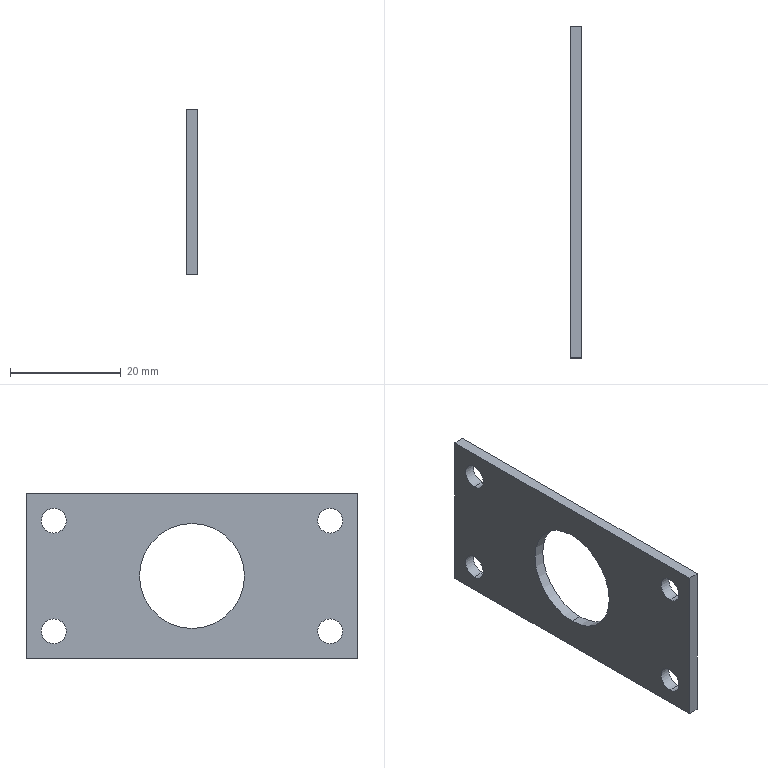Part | STEP file | 06-07 Bearing cover plate | 1 solid | 16 faces | box 2 x 60 x 30 mm | volume 2906 mm3 | cylinder 10 | plane 6 | commonest cylinder face diameters 4.5 x8 19 x2
STEP:
#1=CARTESIAN_POINT('',(0.,0.,0.));
#2=DIRECTION('',(0.,0.,1.));
#3=DIRECTION('',(1.,0.,0.));
#4=AXIS2_PLACEMENT_3D('',#1,#2,#3);
#5=CARTESIAN_POINT('',(2.,-24.996,-7.75));
#6=VERTEX_POINT('',#5);
#7=CARTESIAN_POINT('',(0.,-24.996,-7.75));
#8=VERTEX_POINT('',#7);
#9=CARTESIAN_POINT('',(2.,-24.996,-7.75));
#10=DIRECTION('',(-1.,0.,0.));
#11=VECTOR('',#10,1.);
#12=LINE('',#9,#11);
#13=CARTESIAN_POINT('',(2.,-24.996,-10.));
#14=DIRECTION('',(-1.,0.,0.));
#15=DIRECTION('',(0.,0.,1.));
#16=AXIS2_PLACEMENT_3D('',#13,#14,#15);
#17=CYLINDRICAL_SURFACE('',#16,2.25);
#18=CARTESIAN_POINT('',(6.283,0.));
#19=DIRECTION('',(0.,1.));
#20=VECTOR('',#19,1.);
#21=LINE('',#18,#20);
#22=(GEOMETRIC_REPRESENTATION_CONTEXT(2)PARAMETRIC_REPRESENTATION_CONTEXT()REPRESENTATION_CONTEXT('',''));
#23=DEFINITIONAL_REPRESENTATION('',(#21),#22);
#24=PCURVE('',#17,#23);
#25=CARTESIAN_POINT('',(2.,-24.996,-10.));
#26=DIRECTION('',(-1.,0.,0.));
#27=DIRECTION('',(0.,0.,1.));
#28=AXIS2_PLACEMENT_3D('',#25,#26,#27);
#29=CYLINDRICAL_SURFACE('',#28,2.25);
#30=CARTESIAN_POINT('',(0.,0.));
#31=DIRECTION('',(0.,1.));
#32=VECTOR('',#31,1.);
#33=LINE('',#30,#32);
#34=(GEOMETRIC_REPRESENTATION_CONTEXT(2)PARAMETRIC_REPRESENTATION_CONTEXT()REPRESENTATION_CONTEXT('',''));
#35=DEFINITIONAL_REPRESENTATION('',(#33),#34);
#36=PCURVE('',#29,#35);
#37=SURFACE_CURVE('',#12,(#24,#36),.PCURVE_S1.);
#38=EDGE_CURVE('',#6,#8,#37,.T.);
#39=ORIENTED_EDGE('',*,*,#38,.T.);
#40=CARTESIAN_POINT('',(0.,-24.996,-12.25));
#41=VERTEX_POINT('',#40);
#42=CARTESIAN_POINT('',(0.,-24.996,-10.));
#43=DIRECTION('',(-1.,0.,0.));
#44=DIRECTION('',(0.,0.,1.));
#45=AXIS2_PLACEMENT_3D('',#42,#43,#44);
#46=CIRCLE('',#45,2.25);
#47=CARTESIAN_POINT('',(0.,2.));
#48=DIRECTION('',(1.,0.));
#49=VECTOR('',#48,1.);
#50=LINE('',#47,#49);
#51=(GEOMETRIC_REPRESENTATION_CONTEXT(2)PARAMETRIC_REPRESENTATION_CONTEXT()REPRESENTATION_CONTEXT('',''));
#52=DEFINITIONAL_REPRESENTATION('',(#50),#51);
#53=PCURVE('',#17,#52);
#54=CARTESIAN_POINT('',(0.,-30.,15.));
#55=DIRECTION('',(1.,0.,0.));
#56=DIRECTION('',(0.,0.,-1.));
#57=AXIS2_PLACEMENT_3D('',#54,#55,#56);
#58=PLANE('',#57);
#59=CARTESIAN_POINT('',(22.75,5.004));
#60=CARTESIAN_POINT('',(22.75,8.901));
#61=CARTESIAN_POINT('',(26.125,6.952));
#62=CARTESIAN_POINT('',(29.5,5.004));
#63=CARTESIAN_POINT('',(26.125,3.055));
#64=CARTESIAN_POINT('',(22.75,1.107));
#65=CARTESIAN_POINT('',(22.75,5.004));
#66=(BOUNDED_CURVE()B_SPLINE_CURVE(2,(#59,#60,#61,#62,#63,#64,#65),.UNSPECIFIED.,.T.,.F.)B_SPLINE_CURVE_WITH_KNOTS((1,2,2,2,2,1),(-2.094,0.,2.094,4.189,6.283,8.378),.UNSPECIFIED.)CURVE()GEOMETRIC_REPRESENTATION_ITEM()RATIONAL_B_SPLINE_CURVE((1.,0.5,1.,0.5,1.,0.5,1.))REPRESENTATION_ITEM(''));
#67=(GEOMETRIC_REPRESENTATION_CONTEXT(2)PARAMETRIC_REPRESENTATION_CONTEXT()REPRESENTATION_CONTEXT('',''));
#68=DEFINITIONAL_REPRESENTATION('',(#66),#67);
#69=PCURVE('',#58,#68);
#70=SURFACE_CURVE('',#46,(#53,#69),.PCURVE_S1.);
#71=EDGE_CURVE('',#41,#8,#70,.T.);
#72=ORIENTED_EDGE('',*,*,#71,.F.);
#73=CARTESIAN_POINT('',(2.,-24.996,-12.25));
#74=VERTEX_POINT('',#73);
#75=CARTESIAN_POINT('',(2.,-24.996,-12.25));
#76=DIRECTION('',(-1.,0.,0.));
#77=VECTOR('',#76,1.);
#78=LINE('',#75,#77);
#79=CARTESIAN_POINT('',(3.142,0.));
#80=DIRECTION('',(0.,1.));
#81=VECTOR('',#80,1.);
#82=LINE('',#79,#81);
#83=(GEOMETRIC_REPRESENTATION_CONTEXT(2)PARAMETRIC_REPRESENTATION_CONTEXT()REPRESENTATION_CONTEXT('',''));
#84=DEFINITIONAL_REPRESENTATION('',(#82),#83);
#85=PCURVE('',#17,#84);
#86=CARTESIAN_POINT('',(3.142,0.));
#87=DIRECTION('',(0.,1.));
#88=VECTOR('',#87,1.);
#89=LINE('',#86,#88);
#90=(GEOMETRIC_REPRESENTATION_CONTEXT(2)PARAMETRIC_REPRESENTATION_CONTEXT()REPRESENTATION_CONTEXT('',''));
#91=DEFINITIONAL_REPRESENTATION('',(#89),#90);
#92=PCURVE('',#29,#91);
#93=SURFACE_CURVE('',#78,(#85,#92),.PCURVE_S1.);
#94=EDGE_CURVE('',#74,#41,#93,.T.);
#95=ORIENTED_EDGE('',*,*,#94,.F.);
#96=CARTESIAN_POINT('',(2.,-24.996,-10.));
#97=DIRECTION('',(1.,0.,0.));
#98=DIRECTION('',(0.,0.,1.));
#99=AXIS2_PLACEMENT_3D('',#96,#97,#98);
#100=CIRCLE('',#99,2.25);
#101=CARTESIAN_POINT('',(6.283,0.));
#102=DIRECTION('',(-1.,0.));
#103=VECTOR('',#102,1.);
#104=LINE('',#101,#103);
#105=(GEOMETRIC_REPRESENTATION_CONTEXT(2)PARAMETRIC_REPRESENTATION_CONTEXT()REPRESENTATION_CONTEXT('',''));
#106=DEFINITIONAL_REPRESENTATION('',(#104),#105);
#107=PCURVE('',#17,#106);
#108=CARTESIAN_POINT('',(2.,-30.,15.));
#109=DIRECTION('',(1.,0.,0.));
#110=DIRECTION('',(0.,0.,-1.));
#111=AXIS2_PLACEMENT_3D('',#108,#109,#110);
#112=PLANE('',#111);
#113=CARTESIAN_POINT('',(25.,5.004));
#114=DIRECTION('',(-1.,0.));
#115=AXIS2_PLACEMENT_2D('',#113,#114);
#116=CIRCLE('',#115,2.25);
#117=(GEOMETRIC_REPRESENTATION_CONTEXT(2)PARAMETRIC_REPRESENTATION_CONTEXT()REPRESENTATION_CONTEXT('',''));
#118=DEFINITIONAL_REPRESENTATION('',(#116),#117);
#119=PCURVE('',#112,#118);
#120=SURFACE_CURVE('',#100,(#107,#119),.PCURVE_S1.);
#121=EDGE_CURVE('',#6,#74,#120,.T.);
#122=ORIENTED_EDGE('',*,*,#121,.F.);
#123=EDGE_LOOP('',(#39,#72,#95,#122));
#124=FACE_BOUND('',#123,.F.);
#125=ADVANCED_FACE('',(#124),#17,.F.);
#126=CARTESIAN_POINT('',(2.,25.004,-7.75));
#127=VERTEX_POINT('',#126);
#128=CARTESIAN_POINT('',(0.,25.004,-7.75));
#129=VERTEX_POINT('',#128);
#130=CARTESIAN_POINT('',(2.,25.004,-7.75));
#131=DIRECTION('',(-1.,0.,0.));
#132=VECTOR('',#131,1.);
#133=LINE('',#130,#132);
#134=CARTESIAN_POINT('',(2.,25.004,-10.));
#135=DIRECTION('',(-1.,0.,0.));
#136=DIRECTION('',(0.,0.,1.));
#137=AXIS2_PLACEMENT_3D('',#134,#135,#136);
#138=CYLINDRICAL_SURFACE('',#137,2.25);
#139=CARTESIAN_POINT('',(6.283,0.));
#140=DIRECTION('',(0.,1.));
#141=VECTOR('',#140,1.);
#142=LINE('',#139,#141);
#143=(GEOMETRIC_REPRESENTATION_CONTEXT(2)PARAMETRIC_REPRESENTATION_CONTEXT()REPRESENTATION_CONTEXT('',''));
#144=DEFINITIONAL_REPRESENTATION('',(#142),#143);
#145=PCURVE('',#138,#144);
#146=CARTESIAN_POINT('',(2.,25.004,-10.));
#147=DIRECTION('',(-1.,0.,0.));
#148=DIRECTION('',(0.,0.,1.));
#149=AXIS2_PLACEMENT_3D('',#146,#147,#148);
#150=CYLINDRICAL_SURFACE('',#149,2.25);
#151=CARTESIAN_POINT('',(0.,0.));
#152=DIRECTION('',(0.,1.));
#153=VECTOR('',#152,1.);
#154=LINE('',#151,#153);
#155=(GEOMETRIC_REPRESENTATION_CONTEXT(2)PARAMETRIC_REPRESENTATION_CONTEXT()REPRESENTATION_CONTEXT('',''));
#156=DEFINITIONAL_REPRESENTATION('',(#154),#155);
#157=PCURVE('',#150,#156);
#158=SURFACE_CURVE('',#133,(#145,#157),.PCURVE_S1.);
#159=EDGE_CURVE('',#127,#129,#158,.T.);
#160=ORIENTED_EDGE('',*,*,#159,.T.);
#161=CARTESIAN_POINT('',(0.,25.004,-12.25));
#162=VERTEX_POINT('',#161);
#163=CARTESIAN_POINT('',(0.,25.004,-10.));
#164=DIRECTION('',(-1.,0.,0.));
#165=DIRECTION('',(0.,0.,1.));
#166=AXIS2_PLACEMENT_3D('',#163,#164,#165);
#167=CIRCLE('',#166,2.25);
#168=CARTESIAN_POINT('',(0.,2.));
#169=DIRECTION('',(1.,0.));
#170=VECTOR('',#169,1.);
#171=LINE('',#168,#170);
#172=(GEOMETRIC_REPRESENTATION_CONTEXT(2)PARAMETRIC_REPRESENTATION_CONTEXT()REPRESENTATION_CONTEXT('',''));
#173=DEFINITIONAL_REPRESENTATION('',(#171),#172);
#174=PCURVE('',#138,#173);
#175=CARTESIAN_POINT('',(22.75,55.004));
#176=CARTESIAN_POINT('',(22.75,58.901));
#177=CARTESIAN_POINT('',(26.125,56.952));
#178=CARTESIAN_POINT('',(29.5,55.004));
#179=CARTESIAN_POINT('',(26.125,53.055));
#180=CARTESIAN_POINT('',(22.75,51.107));
#181=CARTESIAN_POINT('',(22.75,55.004));
#182=(BOUNDED_CURVE()B_SPLINE_CURVE(2,(#175,#176,#177,#178,#179,#180,#181),.UNSPECIFIED.,.T.,.F.)B_SPLINE_CURVE_WITH_KNOTS((1,2,2,2,2,1),(-2.094,0.,2.094,4.189,6.283,8.378),.UNSPECIFIED.)CURVE()GEOMETRIC_REPRESENTATION_ITEM()RATIONAL_B_SPLINE_CURVE((1.,0.5,1.,0.5,1.,0.5,1.))REPRESENTATION_ITEM(''));
#183=(GEOMETRIC_REPRESENTATION_CONTEXT(2)PARAMETRIC_REPRESENTATION_CONTEXT()REPRESENTATION_CONTEXT('',''));
#184=DEFINITIONAL_REPRESENTATION('',(#182),#183);
#185=PCURVE('',#58,#184);
#186=SURFACE_CURVE('',#167,(#174,#185),.PCURVE_S1.);
#187=EDGE_CURVE('',#162,#129,#186,.T.);
#188=ORIENTED_EDGE('',*,*,#187,.F.);
#189=CARTESIAN_POINT('',(2.,25.004,-12.25));
#190=VERTEX_POINT('',#189);
#191=CARTESIAN_POINT('',(2.,25.004,-12.25));
#192=DIRECTION('',(-1.,0.,0.));
#193=VECTOR('',#192,1.);
#194=LINE('',#191,#193);
#195=CARTESIAN_POINT('',(3.142,0.));
#196=DIRECTION('',(0.,1.));
#197=VECTOR('',#196,1.);
#198=LINE('',#195,#197);
#199=(GEOMETRIC_REPRESENTATION_CONTEXT(2)PARAMETRIC_REPRESENTATION_CONTEXT()REPRESENTATION_CONTEXT('',''));
#200=DEFINITIONAL_REPRESENTATION('',(#198),#199);
#201=PCURVE('',#138,#200);
#202=CARTESIAN_POINT('',(3.142,0.));
#203=DIRECTION('',(0.,1.));
#204=VECTOR('',#203,1.);
#205=LINE('',#202,#204);
#206=(GEOMETRIC_REPRESENTATION_CONTEXT(2)PARAMETRIC_REPRESENTATION_CONTEXT()REPRESENTATION_CONTEXT('',''));
#207=DEFINITIONAL_REPRESENTATION('',(#205),#206);
#208=PCURVE('',#150,#207);
#209=SURFACE_CURVE('',#194,(#201,#208),.PCURVE_S1.);
#210=EDGE_CURVE('',#190,#162,#209,.T.);
#211=ORIENTED_EDGE('',*,*,#210,.F.);
#212=CARTESIAN_POINT('',(2.,25.004,-10.));
#213=DIRECTION('',(-1.,0.,0.));
#214=DIRECTION('',(0.,0.,1.));
#215=AXIS2_PLACEMENT_3D('',#212,#213,#214);
#216=CIRCLE('',#215,2.25);
#217=CARTESIAN_POINT('',(0.,0.));
#218=DIRECTION('',(1.,0.));
#219=VECTOR('',#218,1.);
#220=LINE('',#217,#219);
#221=(GEOMETRIC_REPRESENTATION_CONTEXT(2)PARAMETRIC_REPRESENTATION_CONTEXT()REPRESENTATION_CONTEXT('',''));
#222=DEFINITIONAL_REPRESENTATION('',(#220),#221);
#223=PCURVE('',#138,#222);
#224=CARTESIAN_POINT('',(22.75,55.004));
#225=CARTESIAN_POINT('',(22.75,58.901));
#226=CARTESIAN_POINT('',(26.125,56.952));
#227=CARTESIAN_POINT('',(29.5,55.004));
#228=CARTESIAN_POINT('',(26.125,53.055));
#229=CARTESIAN_POINT('',(22.75,51.107));
#230=CARTESIAN_POINT('',(22.75,55.004));
#231=(BOUNDED_CURVE()B_SPLINE_CURVE(2,(#224,#225,#226,#227,#228,#229,#230),.UNSPECIFIED.,.T.,.F.)B_SPLINE_CURVE_WITH_KNOTS((1,2,2,2,2,1),(-2.094,0.,2.094,4.189,6.283,8.378),.UNSPECIFIED.)CURVE()GEOMETRIC_REPRESENTATION_ITEM()RATIONAL_B_SPLINE_CURVE((1.,0.5,1.,0.5,1.,0.5,1.))REPRESENTATION_ITEM(''));
#232=(GEOMETRIC_REPRESENTATION_CONTEXT(2)PARAMETRIC_REPRESENTATION_CONTEXT()REPRESENTATION_CONTEXT('',''));
#233=DEFINITIONAL_REPRESENTATION('',(#231),#232);
#234=PCURVE('',#112,#233);
#235=SURFACE_CURVE('',#216,(#223,#234),.PCURVE_S1.);
#236=EDGE_CURVE('',#190,#127,#235,.T.);
#237=ORIENTED_EDGE('',*,*,#236,.T.);
#238=EDGE_LOOP('',(#160,#188,#211,#237));
#239=FACE_BOUND('',#238,.F.);
#240=ADVANCED_FACE('',(#239),#138,.F.);
#241=CARTESIAN_POINT('',(2.,0.,9.5));
#242=VERTEX_POINT('',#241);
#243=CARTESIAN_POINT('',(0.,0.,9.5));
#244=VERTEX_POINT('',#243);
#245=CARTESIAN_POINT('',(2.,0.,9.5));
#246=DIRECTION('',(-1.,0.,0.));
#247=VECTOR('',#246,1.);
#248=LINE('',#245,#247);
#249=CARTESIAN_POINT('',(2.,0.,0.));
#250=DIRECTION('',(-1.,0.,0.));
#251=DIRECTION('',(0.,0.,1.));
#252=AXIS2_PLACEMENT_3D('',#249,#250,#251);
#253=CYLINDRICAL_SURFACE('',#252,9.5);
#254=CARTESIAN_POINT('',(6.283,0.));
#255=DIRECTION('',(0.,1.));
#256=VECTOR('',#255,1.);
#257=LINE('',#254,#256);
#258=(GEOMETRIC_REPRESENTATION_CONTEXT(2)PARAMETRIC_REPRESENTATION_CONTEXT()REPRESENTATION_CONTEXT('',''));
#259=DEFINITIONAL_REPRESENTATION('',(#257),#258);
#260=PCURVE('',#253,#259);
#261=CARTESIAN_POINT('',(2.,0.,0.));
#262=DIRECTION('',(-1.,0.,0.));
#263=DIRECTION('',(0.,0.,1.));
#264=AXIS2_PLACEMENT_3D('',#261,#262,#263);
#265=CYLINDRICAL_SURFACE('',#264,9.5);
#266=CARTESIAN_POINT('',(0.,0.));
#267=DIRECTION('',(0.,1.));
#268=VECTOR('',#267,1.);
#269=LINE('',#266,#268);
#270=(GEOMETRIC_REPRESENTATION_CONTEXT(2)PARAMETRIC_REPRESENTATION_CONTEXT()REPRESENTATION_CONTEXT('',''));
#271=DEFINITIONAL_REPRESENTATION('',(#269),#270);
#272=PCURVE('',#265,#271);
#273=SURFACE_CURVE('',#248,(#260,#272),.PCURVE_S1.);
#274=EDGE_CURVE('',#242,#244,#273,.T.);
#275=ORIENTED_EDGE('',*,*,#274,.T.);
#276=CARTESIAN_POINT('',(0.,0.,-9.5));
#277=VERTEX_POINT('',#276);
#278=CARTESIAN_POINT('',(0.,0.,0.));
#279=DIRECTION('',(-1.,0.,0.));
#280=DIRECTION('',(0.,0.,1.));
#281=AXIS2_PLACEMENT_3D('',#278,#279,#280);
#282=CIRCLE('',#281,9.5);
#283=CARTESIAN_POINT('',(0.,2.));
#284=DIRECTION('',(1.,0.));
#285=VECTOR('',#284,1.);
#286=LINE('',#283,#285);
#287=(GEOMETRIC_REPRESENTATION_CONTEXT(2)PARAMETRIC_REPRESENTATION_CONTEXT()REPRESENTATION_CONTEXT('',''));
#288=DEFINITIONAL_REPRESENTATION('',(#286),#287);
#289=PCURVE('',#253,#288);
#290=CARTESIAN_POINT('',(5.5,30.));
#291=CARTESIAN_POINT('',(5.5,46.454));
#292=CARTESIAN_POINT('',(19.75,38.227));
#293=CARTESIAN_POINT('',(34.,30.));
#294=CARTESIAN_POINT('',(19.75,21.773));
#295=CARTESIAN_POINT('',(5.5,13.546));
#296=CARTESIAN_POINT('',(5.5,30.));
#297=(BOUNDED_CURVE()B_SPLINE_CURVE(2,(#290,#291,#292,#293,#294,#295,#296),.UNSPECIFIED.,.T.,.F.)B_SPLINE_CURVE_WITH_KNOTS((1,2,2,2,2,1),(-2.094,0.,2.094,4.189,6.283,8.378),.UNSPECIFIED.)CURVE()GEOMETRIC_REPRESENTATION_ITEM()RATIONAL_B_SPLINE_CURVE((1.,0.5,1.,0.5,1.,0.5,1.))REPRESENTATION_ITEM(''));
#298=(GEOMETRIC_REPRESENTATION_CONTEXT(2)PARAMETRIC_REPRESENTATION_CONTEXT()REPRESENTATION_CONTEXT('',''));
#299=DEFINITIONAL_REPRESENTATION('',(#297),#298);
#300=PCURVE('',#58,#299);
#301=SURFACE_CURVE('',#282,(#289,#300),.PCURVE_S1.);
#302=EDGE_CURVE('',#277,#244,#301,.T.);
#303=ORIENTED_EDGE('',*,*,#302,.F.);
#304=CARTESIAN_POINT('',(2.,0.,-9.5));
#305=VERTEX_POINT('',#304);
#306=CARTESIAN_POINT('',(2.,0.,-9.5));
#307=DIRECTION('',(-1.,0.,0.));
#308=VECTOR('',#307,1.);
#309=LINE('',#306,#308);
#310=CARTESIAN_POINT('',(3.142,0.));
#311=DIRECTION('',(0.,1.));
#312=VECTOR('',#311,1.);
#313=LINE('',#310,#312);
#314=(GEOMETRIC_REPRESENTATION_CONTEXT(2)PARAMETRIC_REPRESENTATION_CONTEXT()REPRESENTATION_CONTEXT('',''));
#315=DEFINITIONAL_REPRESENTATION('',(#313),#314);
#316=PCURVE('',#253,#315);
#317=CARTESIAN_POINT('',(3.142,0.));
#318=DIRECTION('',(0.,1.));
#319=VECTOR('',#318,1.);
#320=LINE('',#317,#319);
#321=(GEOMETRIC_REPRESENTATION_CONTEXT(2)PARAMETRIC_REPRESENTATION_CONTEXT()REPRESENTATION_CONTEXT('',''));
#322=DEFINITIONAL_REPRESENTATION('',(#320),#321);
#323=PCURVE('',#265,#322);
#324=SURFACE_CURVE('',#309,(#316,#323),.PCURVE_S1.);
#325=EDGE_CURVE('',#305,#277,#324,.T.);
#326=ORIENTED_EDGE('',*,*,#325,.F.);
#327=CARTESIAN_POINT('',(2.,0.,0.));
#328=DIRECTION('',(-1.,0.,0.));
#329=DIRECTION('',(0.,0.,1.));
#330=AXIS2_PLACEMENT_3D('',#327,#328,#329);
#331=CIRCLE('',#330,9.5);
#332=CARTESIAN_POINT('',(0.,0.));
#333=DIRECTION('',(1.,0.));
#334=VECTOR('',#333,1.);
#335=LINE('',#332,#334);
#336=(GEOMETRIC_REPRESENTATION_CONTEXT(2)PARAMETRIC_REPRESENTATION_CONTEXT()REPRESENTATION_CONTEXT('',''));
#337=DEFINITIONAL_REPRESENTATION('',(#335),#336);
#338=PCURVE('',#253,#337);
#339=CARTESIAN_POINT('',(5.5,30.));
#340=CARTESIAN_POINT('',(5.5,46.454));
#341=CARTESIAN_POINT('',(19.75,38.227));
#342=CARTESIAN_POINT('',(34.,30.));
#343=CARTESIAN_POINT('',(19.75,21.773));
#344=CARTESIAN_POINT('',(5.5,13.546));
#345=CARTESIAN_POINT('',(5.5,30.));
#346=(BOUNDED_CURVE()B_SPLINE_CURVE(2,(#339,#340,#341,#342,#343,#344,#345),.UNSPECIFIED.,.T.,.F.)B_SPLINE_CURVE_WITH_KNOTS((1,2,2,2,2,1),(-2.094,0.,2.094,4.189,6.283,8.378),.UNSPECIFIED.)CURVE()GEOMETRIC_REPRESENTATION_ITEM()RATIONAL_B_SPLINE_CURVE((1.,0.5,1.,0.5,1.,0.5,1.))REPRESENTATION_ITEM(''));
#347=(GEOMETRIC_REPRESENTATION_CONTEXT(2)PARAMETRIC_REPRESENTATION_CONTEXT()REPRESENTATION_CONTEXT('',''));
#348=DEFINITIONAL_REPRESENTATION('',(#346),#347);
#349=PCURVE('',#112,#348);
#350=SURFACE_CURVE('',#331,(#338,#349),.PCURVE_S1.);
#351=EDGE_CURVE('',#305,#242,#350,.T.);
#352=ORIENTED_EDGE('',*,*,#351,.T.);
#353=EDGE_LOOP('',(#275,#303,#326,#352));
#354=FACE_BOUND('',#353,.F.);
#355=ADVANCED_FACE('',(#354),#253,.F.);
#356=CARTESIAN_POINT('',(2.,25.004,12.25));
#357=VERTEX_POINT('',#356);
#358=CARTESIAN_POINT('',(0.,25.004,12.25));
#359=VERTEX_POINT('',#358);
#360=CARTESIAN_POINT('',(2.,25.004,12.25));
#361=DIRECTION('',(-1.,0.,0.));
#362=VECTOR('',#361,1.);
#363=LINE('',#360,#362);
#364=CARTESIAN_POINT('',(2.,25.004,10.));
#365=DIRECTION('',(-1.,0.,0.));
#366=DIRECTION('',(0.,0.,1.));
#367=AXIS2_PLACEMENT_3D('',#364,#365,#366);
#368=CYLINDRICAL_SURFACE('',#367,2.25);
#369=CARTESIAN_POINT('',(6.283,0.));
#370=DIRECTION('',(0.,1.));
#371=VECTOR('',#370,1.);
#372=LINE('',#369,#371);
#373=(GEOMETRIC_REPRESENTATION_CONTEXT(2)PARAMETRIC_REPRESENTATION_CONTEXT()REPRESENTATION_CONTEXT('',''));
#374=DEFINITIONAL_REPRESENTATION('',(#372),#373);
#375=PCURVE('',#368,#374);
#376=CARTESIAN_POINT('',(2.,25.004,10.));
#377=DIRECTION('',(-1.,0.,0.));
#378=DIRECTION('',(0.,0.,1.));
#379=AXIS2_PLACEMENT_3D('',#376,#377,#378);
#380=CYLINDRICAL_SURFACE('',#379,2.25);
#381=CARTESIAN_POINT('',(0.,0.));
#382=DIRECTION('',(0.,1.));
#383=VECTOR('',#382,1.);
#384=LINE('',#381,#383);
#385=(GEOMETRIC_REPRESENTATION_CONTEXT(2)PARAMETRIC_REPRESENTATION_CONTEXT()REPRESENTATION_CONTEXT('',''));
#386=DEFINITIONAL_REPRESENTATION('',(#384),#385);
#387=PCURVE('',#380,#386);
#388=SURFACE_CURVE('',#363,(#375,#387),.PCURVE_S1.);
#389=EDGE_CURVE('',#357,#359,#388,.T.);
#390=ORIENTED_EDGE('',*,*,#389,.T.);
#391=CARTESIAN_POINT('',(0.,25.004,7.75));
#392=VERTEX_POINT('',#391);
#393=CARTESIAN_POINT('',(0.,25.004,10.));
#394=DIRECTION('',(-1.,0.,0.));
#395=DIRECTION('',(0.,0.,1.));
#396=AXIS2_PLACEMENT_3D('',#393,#394,#395);
#397=CIRCLE('',#396,2.25);
#398=CARTESIAN_POINT('',(0.,2.));
#399=DIRECTION('',(1.,0.));
#400=VECTOR('',#399,1.);
#401=LINE('',#398,#400);
#402=(GEOMETRIC_REPRESENTATION_CONTEXT(2)PARAMETRIC_REPRESENTATION_CONTEXT()REPRESENTATION_CONTEXT('',''));
#403=DEFINITIONAL_REPRESENTATION('',(#401),#402);
#404=PCURVE('',#368,#403);
#405=CARTESIAN_POINT('',(2.75,55.004));
#406=CARTESIAN_POINT('',(2.75,58.901));
#407=CARTESIAN_POINT('',(6.125,56.952));
#408=CARTESIAN_POINT('',(9.5,55.004));
#409=CARTESIAN_POINT('',(6.125,53.055));
#410=CARTESIAN_POINT('',(2.75,51.107));
#411=CARTESIAN_POINT('',(2.75,55.004));
#412=(BOUNDED_CURVE()B_SPLINE_CURVE(2,(#405,#406,#407,#408,#409,#410,#411),.UNSPECIFIED.,.T.,.F.)B_SPLINE_CURVE_WITH_KNOTS((1,2,2,2,2,1),(-2.094,0.,2.094,4.189,6.283,8.378),.UNSPECIFIED.)CURVE()GEOMETRIC_REPRESENTATION_ITEM()RATIONAL_B_SPLINE_CURVE((1.,0.5,1.,0.5,1.,0.5,1.))REPRESENTATION_ITEM(''));
#413=(GEOMETRIC_REPRESENTATION_CONTEXT(2)PARAMETRIC_REPRESENTATION_CONTEXT()REPRESENTATION_CONTEXT('',''));
#414=DEFINITIONAL_REPRESENTATION('',(#412),#413);
#415=PCURVE('',#58,#414);
#416=SURFACE_CURVE('',#397,(#404,#415),.PCURVE_S1.);
#417=EDGE_CURVE('',#392,#359,#416,.T.);
#418=ORIENTED_EDGE('',*,*,#417,.F.);
#419=CARTESIAN_POINT('',(2.,25.004,7.75));
#420=VERTEX_POINT('',#419);
#421=CARTESIAN_POINT('',(2.,25.004,7.75));
#422=DIRECTION('',(-1.,0.,0.));
#423=VECTOR('',#422,1.);
#424=LINE('',#421,#423);
#425=CARTESIAN_POINT('',(3.142,0.));
#426=DIRECTION('',(0.,1.));
#427=VECTOR('',#426,1.);
#428=LINE('',#425,#427);
#429=(GEOMETRIC_REPRESENTATION_CONTEXT(2)PARAMETRIC_REPRESENTATION_CONTEXT()REPRESENTATION_CONTEXT('',''));
#430=DEFINITIONAL_REPRESENTATION('',(#428),#429);
#431=PCURVE('',#368,#430);
#432=CARTESIAN_POINT('',(3.142,0.));
#433=DIRECTION('',(0.,1.));
#434=VECTOR('',#433,1.);
#435=LINE('',#432,#434);
#436=(GEOMETRIC_REPRESENTATION_CONTEXT(2)PARAMETRIC_REPRESENTATION_CONTEXT()REPRESENTATION_CONTEXT('',''));
#437=DEFINITIONAL_REPRESENTATION('',(#435),#436);
#438=PCURVE('',#380,#437);
#439=SURFACE_CURVE('',#424,(#431,#438),.PCURVE_S1.);
#440=EDGE_CURVE('',#420,#392,#439,.T.);
#441=ORIENTED_EDGE('',*,*,#440,.F.);
#442=CARTESIAN_POINT('',(2.,25.004,10.));
#443=DIRECTION('',(-1.,0.,0.));
#444=DIRECTION('',(0.,0.,1.));
#445=AXIS2_PLACEMENT_3D('',#442,#443,#444);
#446=CIRCLE('',#445,2.25);
#447=CARTESIAN_POINT('',(0.,0.));
#448=DIRECTION('',(1.,0.));
#449=VECTOR('',#448,1.);
#450=LINE('',#447,#449);
#451=(GEOMETRIC_REPRESENTATION_CONTEXT(2)PARAMETRIC_REPRESENTATION_CONTEXT()REPRESENTATION_CONTEXT('',''));
#452=DEFINITIONAL_REPRESENTATION('',(#450),#451);
#453=PCURVE('',#368,#452);
#454=CARTESIAN_POINT('',(2.75,55.004));
#455=CARTESIAN_POINT('',(2.75,58.901));
#456=CARTESIAN_POINT('',(6.125,56.952));
#457=CARTESIAN_POINT('',(9.5,55.004));
#458=CARTESIAN_POINT('',(6.125,53.055));
#459=CARTESIAN_POINT('',(2.75,51.107));
#460=CARTESIAN_POINT('',(2.75,55.004));
#461=(BOUNDED_CURVE()B_SPLINE_CURVE(2,(#454,#455,#456,#457,#458,#459,#460),.UNSPECIFIED.,.T.,.F.)B_SPLINE_CURVE_WITH_KNOTS((1,2,2,2,2,1),(-2.094,0.,2.094,4.189,6.283,8.378),.UNSPECIFIED.)CURVE()GEOMETRIC_REPRESENTATION_ITEM()RATIONAL_B_SPLINE_CURVE((1.,0.5,1.,0.5,1.,0.5,1.))REPRESENTATION_ITEM(''));
#462=(GEOMETRIC_REPRESENTATION_CONTEXT(2)PARAMETRIC_REPRESENTATION_CONTEXT()REPRESENTATION_CONTEXT('',''));
#463=DEFINITIONAL_REPRESENTATION('',(#461),#462);
#464=PCURVE('',#112,#463);
#465=SURFACE_CURVE('',#446,(#453,#464),.PCURVE_S1.);
#466=EDGE_CURVE('',#420,#357,#465,.T.);
#467=ORIENTED_EDGE('',*,*,#466,.T.);
#468=EDGE_LOOP('',(#390,#418,#441,#467));
#469=FACE_BOUND('',#468,.F.);
#470=ADVANCED_FACE('',(#469),#368,.F.);
#471=CARTESIAN_POINT('',(2.,-24.996,12.25));
#472=VERTEX_POINT('',#471);
#473=CARTESIAN_POINT('',(0.,-24.996,12.25));
#474=VERTEX_POINT('',#473);
#475=CARTESIAN_POINT('',(2.,-24.996,12.25));
#476=DIRECTION('',(-1.,0.,0.));
#477=VECTOR('',#476,1.);
#478=LINE('',#475,#477);
#479=CARTESIAN_POINT('',(2.,-24.996,10.));
#480=DIRECTION('',(-1.,0.,0.));
#481=DIRECTION('',(0.,0.,1.));
#482=AXIS2_PLACEMENT_3D('',#479,#480,#481);
#483=CYLINDRICAL_SURFACE('',#482,2.25);
#484=CARTESIAN_POINT('',(6.283,0.));
#485=DIRECTION('',(0.,1.));
#486=VECTOR('',#485,1.);
#487=LINE('',#484,#486);
#488=(GEOMETRIC_REPRESENTATION_CONTEXT(2)PARAMETRIC_REPRESENTATION_CONTEXT()REPRESENTATION_CONTEXT('',''));
#489=DEFINITIONAL_REPRESENTATION('',(#487),#488);
#490=PCURVE('',#483,#489);
#491=CARTESIAN_POINT('',(2.,-24.996,10.));
#492=DIRECTION('',(-1.,0.,0.));
#493=DIRECTION('',(0.,0.,1.));
#494=AXIS2_PLACEMENT_3D('',#491,#492,#493);
#495=CYLINDRICAL_SURFACE('',#494,2.25);
#496=CARTESIAN_POINT('',(0.,0.));
#497=DIRECTION('',(0.,1.));
#498=VECTOR('',#497,1.);
#499=LINE('',#496,#498);
#500=(GEOMETRIC_REPRESENTATION_CONTEXT(2)PARAMETRIC_REPRESENTATION_CONTEXT()REPRESENTATION_CONTEXT('',''));
#501=DEFINITIONAL_REPRESENTATION('',(#499),#500);
#502=PCURVE('',#495,#501);
#503=SURFACE_CURVE('',#478,(#490,#502),.PCURVE_S1.);
#504=EDGE_CURVE('',#472,#474,#503,.T.);
#505=ORIENTED_EDGE('',*,*,#504,.T.);
#506=CARTESIAN_POINT('',(0.,-24.996,7.75));
#507=VERTEX_POINT('',#506);
#508=CARTESIAN_POINT('',(0.,-24.996,10.));
#509=DIRECTION('',(-1.,0.,0.));
#510=DIRECTION('',(0.,0.,1.));
#511=AXIS2_PLACEMENT_3D('',#508,#509,#510);
#512=CIRCLE('',#511,2.25);
#513=CARTESIAN_POINT('',(0.,2.));
#514=DIRECTION('',(1.,0.));
#515=VECTOR('',#514,1.);
#516=LINE('',#513,#515);
#517=(GEOMETRIC_REPRESENTATION_CONTEXT(2)PARAMETRIC_REPRESENTATION_CONTEXT()REPRESENTATION_CONTEXT('',''));
#518=DEFINITIONAL_REPRESENTATION('',(#516),#517);
#519=PCURVE('',#483,#518);
#520=CARTESIAN_POINT('',(2.75,5.004));
#521=CARTESIAN_POINT('',(2.75,8.901));
#522=CARTESIAN_POINT('',(6.125,6.952));
#523=CARTESIAN_POINT('',(9.5,5.004));
#524=CARTESIAN_POINT('',(6.125,3.055));
#525=CARTESIAN_POINT('',(2.75,1.107));
#526=CARTESIAN_POINT('',(2.75,5.004));
#527=(BOUNDED_CURVE()B_SPLINE_CURVE(2,(#520,#521,#522,#523,#524,#525,#526),.UNSPECIFIED.,.T.,.F.)B_SPLINE_CURVE_WITH_KNOTS((1,2,2,2,2,1),(-2.094,0.,2.094,4.189,6.283,8.378),.UNSPECIFIED.)CURVE()GEOMETRIC_REPRESENTATION_ITEM()RATIONAL_B_SPLINE_CURVE((1.,0.5,1.,0.5,1.,0.5,1.))REPRESENTATION_ITEM(''));
#528=(GEOMETRIC_REPRESENTATION_CONTEXT(2)PARAMETRIC_REPRESENTATION_CONTEXT()REPRESENTATION_CONTEXT('',''));
#529=DEFINITIONAL_REPRESENTATION('',(#527),#528);
#530=PCURVE('',#58,#529);
#531=SURFACE_CURVE('',#512,(#519,#530),.PCURVE_S1.);
#532=EDGE_CURVE('',#507,#474,#531,.T.);
#533=ORIENTED_EDGE('',*,*,#532,.F.);
#534=CARTESIAN_POINT('',(2.,-24.996,7.75));
#535=VERTEX_POINT('',#534);
#536=CARTESIAN_POINT('',(2.,-24.996,7.75));
#537=DIRECTION('',(-1.,0.,0.));
#538=VECTOR('',#537,1.);
#539=LINE('',#536,#538);
#540=CARTESIAN_POINT('',(3.142,0.));
#541=DIRECTION('',(0.,1.));
#542=VECTOR('',#541,1.);
#543=LINE('',#540,#542);
#544=(GEOMETRIC_REPRESENTATION_CONTEXT(2)PARAMETRIC_REPRESENTATION_CONTEXT()REPRESENTATION_CONTEXT('',''));
#545=DEFINITIONAL_REPRESENTATION('',(#543),#544);
#546=PCURVE('',#483,#545);
#547=CARTESIAN_POINT('',(3.142,0.));
#548=DIRECTION('',(0.,1.));
#549=VECTOR('',#548,1.);
#550=LINE('',#547,#549);
#551=(GEOMETRIC_REPRESENTATION_CONTEXT(2)PARAMETRIC_REPRESENTATION_CONTEXT()REPRESENTATION_CONTEXT('',''));
#552=DEFINITIONAL_REPRESENTATION('',(#550),#551);
#553=PCURVE('',#495,#552);
#554=SURFACE_CURVE('',#539,(#546,#553),.PCURVE_S1.);
#555=EDGE_CURVE('',#535,#507,#554,.T.);
#556=ORIENTED_EDGE('',*,*,#555,.F.);
#557=CARTESIAN_POINT('',(2.,-24.996,10.));
#558=DIRECTION('',(-1.,0.,0.));
#559=DIRECTION('',(0.,0.,1.));
#560=AXIS2_PLACEMENT_3D('',#557,#558,#559);
#561=CIRCLE('',#560,2.25);
#562=CARTESIAN_POINT('',(0.,0.));
#563=DIRECTION('',(1.,0.));
#564=VECTOR('',#563,1.);
#565=LINE('',#562,#564);
#566=(GEOMETRIC_REPRESENTATION_CONTEXT(2)PARAMETRIC_REPRESENTATION_CONTEXT()REPRESENTATION_CONTEXT('',''));
#567=DEFINITIONAL_REPRESENTATION('',(#565),#566);
#568=PCURVE('',#483,#567);
#569=CARTESIAN_POINT('',(2.75,5.004));
#570=CARTESIAN_POINT('',(2.75,8.901));
#571=CARTESIAN_POINT('',(6.125,6.952));
#572=CARTESIAN_POINT('',(9.5,5.004));
#573=CARTESIAN_POINT('',(6.125,3.055));
#574=CARTESIAN_POINT('',(2.75,1.107));
#575=CARTESIAN_POINT('',(2.75,5.004));
#576=(BOUNDED_CURVE()B_SPLINE_CURVE(2,(#569,#570,#571,#572,#573,#574,#575),.UNSPECIFIED.,.T.,.F.)B_SPLINE_CURVE_WITH_KNOTS((1,2,2,2,2,1),(-2.094,0.,2.094,4.189,6.283,8.378),.UNSPECIFIED.)CURVE()GEOMETRIC_REPRESENTATION_ITEM()RATIONAL_B_SPLINE_CURVE((1.,0.5,1.,0.5,1.,0.5,1.))REPRESENTATION_ITEM(''));
#577=(GEOMETRIC_REPRESENTATION_CONTEXT(2)PARAMETRIC_REPRESENTATION_CONTEXT()REPRESENTATION_CONTEXT('',''));
#578=DEFINITIONAL_REPRESENTATION('',(#576),#577);
#579=PCURVE('',#112,#578);
#580=SURFACE_CURVE('',#561,(#568,#579),.PCURVE_S1.);
#581=EDGE_CURVE('',#535,#472,#580,.T.);
#582=ORIENTED_EDGE('',*,*,#581,.T.);
#583=EDGE_LOOP('',(#505,#533,#556,#582));
#584=FACE_BOUND('',#583,.F.);
#585=ADVANCED_FACE('',(#584),#483,.F.);
#586=CARTESIAN_POINT('',(0.,-24.996,-10.));
#587=DIRECTION('',(-1.,0.,0.));
#588=DIRECTION('',(0.,0.,1.));
#589=AXIS2_PLACEMENT_3D('',#586,#587,#588);
#590=CIRCLE('',#589,2.25);
#591=CARTESIAN_POINT('',(0.,2.));
#592=DIRECTION('',(1.,0.));
#593=VECTOR('',#592,1.);
#594=LINE('',#591,#593);
#595=(GEOMETRIC_REPRESENTATION_CONTEXT(2)PARAMETRIC_REPRESENTATION_CONTEXT()REPRESENTATION_CONTEXT('',''));
#596=DEFINITIONAL_REPRESENTATION('',(#594),#595);
#597=PCURVE('',#29,#596);
#598=CARTESIAN_POINT('',(22.75,5.004));
#599=CARTESIAN_POINT('',(22.75,8.901));
#600=CARTESIAN_POINT('',(26.125,6.952));
#601=CARTESIAN_POINT('',(29.5,5.004));
#602=CARTESIAN_POINT('',(26.125,3.055));
#603=CARTESIAN_POINT('',(22.75,1.107));
#604=CARTESIAN_POINT('',(22.75,5.004));
#605=(BOUNDED_CURVE()B_SPLINE_CURVE(2,(#598,#599,#600,#601,#602,#603,#604),.UNSPECIFIED.,.T.,.F.)B_SPLINE_CURVE_WITH_KNOTS((1,2,2,2,2,1),(-2.094,0.,2.094,4.189,6.283,8.378),.UNSPECIFIED.)CURVE()GEOMETRIC_REPRESENTATION_ITEM()RATIONAL_B_SPLINE_CURVE((1.,0.5,1.,0.5,1.,0.5,1.))REPRESENTATION_ITEM(''));
#606=(GEOMETRIC_REPRESENTATION_CONTEXT(2)PARAMETRIC_REPRESENTATION_CONTEXT()REPRESENTATION_CONTEXT('',''));
#607=DEFINITIONAL_REPRESENTATION('',(#605),#606);
#608=PCURVE('',#58,#607);
#609=SURFACE_CURVE('',#590,(#597,#608),.PCURVE_S1.);
#610=EDGE_CURVE('',#8,#41,#609,.T.);
#611=ORIENTED_EDGE('',*,*,#610,.F.);
#612=ORIENTED_EDGE('',*,*,#38,.F.);
#613=CARTESIAN_POINT('',(2.,-24.996,-10.));
#614=DIRECTION('',(1.,0.,0.));
#615=DIRECTION('',(0.,0.,1.));
#616=AXIS2_PLACEMENT_3D('',#613,#614,#615);
#617=CIRCLE('',#616,2.25);
#618=CARTESIAN_POINT('',(6.283,0.));
#619=DIRECTION('',(-1.,0.));
#620=VECTOR('',#619,1.);
#621=LINE('',#618,#620);
#622=(GEOMETRIC_REPRESENTATION_CONTEXT(2)PARAMETRIC_REPRESENTATION_CONTEXT()REPRESENTATION_CONTEXT('',''));
#623=DEFINITIONAL_REPRESENTATION('',(#621),#622);
#624=PCURVE('',#29,#623);
#625=CARTESIAN_POINT('',(25.,5.004));
#626=DIRECTION('',(-1.,0.));
#627=AXIS2_PLACEMENT_2D('',#625,#626);
#628=CIRCLE('',#627,2.25);
#629=(GEOMETRIC_REPRESENTATION_CONTEXT(2)PARAMETRIC_REPRESENTATION_CONTEXT()REPRESENTATION_CONTEXT('',''));
#630=DEFINITIONAL_REPRESENTATION('',(#628),#629);
#631=PCURVE('',#112,#630);
#632=SURFACE_CURVE('',#617,(#624,#631),.PCURVE_S1.);
#633=EDGE_CURVE('',#74,#6,#632,.T.);
#634=ORIENTED_EDGE('',*,*,#633,.F.);
#635=ORIENTED_EDGE('',*,*,#94,.T.);
#636=EDGE_LOOP('',(#611,#612,#634,#635));
#637=FACE_BOUND('',#636,.F.);
#638=ADVANCED_FACE('',(#637),#29,.F.);
#639=ORIENTED_EDGE('',*,*,#610,.F.);
#640=ORIENTED_EDGE('',*,*,#71,.F.);
#641=EDGE_LOOP('',(#639,#640));
#642=FACE_BOUND('',#641,.T.);
#643=CARTESIAN_POINT('',(0.,25.004,-10.));
#644=DIRECTION('',(-1.,0.,0.));
#645=DIRECTION('',(0.,0.,1.));
#646=AXIS2_PLACEMENT_3D('',#643,#644,#645);
#647=CIRCLE('',#646,2.25);
#648=CARTESIAN_POINT('',(22.75,55.004));
#649=CARTESIAN_POINT('',(22.75,58.901));
#650=CARTESIAN_POINT('',(26.125,56.952));
#651=CARTESIAN_POINT('',(29.5,55.004));
#652=CARTESIAN_POINT('',(26.125,53.055));
#653=CARTESIAN_POINT('',(22.75,51.107));
#654=CARTESIAN_POINT('',(22.75,55.004));
#655=(BOUNDED_CURVE()B_SPLINE_CURVE(2,(#648,#649,#650,#651,#652,#653,#654),.UNSPECIFIED.,.T.,.F.)B_SPLINE_CURVE_WITH_KNOTS((1,2,2,2,2,1),(-2.094,0.,2.094,4.189,6.283,8.378),.UNSPECIFIED.)CURVE()GEOMETRIC_REPRESENTATION_ITEM()RATIONAL_B_SPLINE_CURVE((1.,0.5,1.,0.5,1.,0.5,1.))REPRESENTATION_ITEM(''));
#656=(GEOMETRIC_REPRESENTATION_CONTEXT(2)PARAMETRIC_REPRESENTATION_CONTEXT()REPRESENTATION_CONTEXT('',''));
#657=DEFINITIONAL_REPRESENTATION('',(#655),#656);
#658=PCURVE('',#58,#657);
#659=CARTESIAN_POINT('',(0.,2.));
#660=DIRECTION('',(1.,0.));
#661=VECTOR('',#660,1.);
#662=LINE('',#659,#661);
#663=(GEOMETRIC_REPRESENTATION_CONTEXT(2)PARAMETRIC_REPRESENTATION_CONTEXT()REPRESENTATION_CONTEXT('',''));
#664=DEFINITIONAL_REPRESENTATION('',(#662),#663);
#665=PCURVE('',#150,#664);
#666=SURFACE_CURVE('',#647,(#658,#665),.PCURVE_S1.);
#667=EDGE_CURVE('',#129,#162,#666,.T.);
#668=ORIENTED_EDGE('',*,*,#667,.F.);
#669=ORIENTED_EDGE('',*,*,#187,.F.);
#670=EDGE_LOOP('',(#668,#669));
#671=FACE_BOUND('',#670,.T.);
#672=CARTESIAN_POINT('',(0.,0.,0.));
#673=DIRECTION('',(-1.,0.,0.));
#674=DIRECTION('',(0.,0.,1.));
#675=AXIS2_PLACEMENT_3D('',#672,#673,#674);
#676=CIRCLE('',#675,9.5);
#677=CARTESIAN_POINT('',(5.5,30.));
#678=CARTESIAN_POINT('',(5.5,46.454));
#679=CARTESIAN_POINT('',(19.75,38.227));
#680=CARTESIAN_POINT('',(34.,30.));
#681=CARTESIAN_POINT('',(19.75,21.773));
#682=CARTESIAN_POINT('',(5.5,13.546));
#683=CARTESIAN_POINT('',(5.5,30.));
#684=(BOUNDED_CURVE()B_SPLINE_CURVE(2,(#677,#678,#679,#680,#681,#682,#683),.UNSPECIFIED.,.T.,.F.)B_SPLINE_CURVE_WITH_KNOTS((1,2,2,2,2,1),(-2.094,0.,2.094,4.189,6.283,8.378),.UNSPECIFIED.)CURVE()GEOMETRIC_REPRESENTATION_ITEM()RATIONAL_B_SPLINE_CURVE((1.,0.5,1.,0.5,1.,0.5,1.))REPRESENTATION_ITEM(''));
#685=(GEOMETRIC_REPRESENTATION_CONTEXT(2)PARAMETRIC_REPRESENTATION_CONTEXT()REPRESENTATION_CONTEXT('',''));
#686=DEFINITIONAL_REPRESENTATION('',(#684),#685);
#687=PCURVE('',#58,#686);
#688=CARTESIAN_POINT('',(0.,2.));
#689=DIRECTION('',(1.,0.));
#690=VECTOR('',#689,1.);
#691=LINE('',#688,#690);
#692=(GEOMETRIC_REPRESENTATION_CONTEXT(2)PARAMETRIC_REPRESENTATION_CONTEXT()REPRESENTATION_CONTEXT('',''));
#693=DEFINITIONAL_REPRESENTATION('',(#691),#692);
#694=PCURVE('',#265,#693);
#695=SURFACE_CURVE('',#676,(#687,#694),.PCURVE_S1.);
#696=EDGE_CURVE('',#244,#277,#695,.T.);
#697=ORIENTED_EDGE('',*,*,#696,.F.);
#698=ORIENTED_EDGE('',*,*,#302,.F.);
#699=EDGE_LOOP('',(#697,#698));
#700=FACE_BOUND('',#699,.T.);
#701=CARTESIAN_POINT('',(0.,25.004,10.));
#702=DIRECTION('',(-1.,0.,0.));
#703=DIRECTION('',(0.,0.,1.));
#704=AXIS2_PLACEMENT_3D('',#701,#702,#703);
#705=CIRCLE('',#704,2.25);
#706=CARTESIAN_POINT('',(2.75,55.004));
#707=CARTESIAN_POINT('',(2.75,58.901));
#708=CARTESIAN_POINT('',(6.125,56.952));
#709=CARTESIAN_POINT('',(9.5,55.004));
#710=CARTESIAN_POINT('',(6.125,53.055));
#711=CARTESIAN_POINT('',(2.75,51.107));
#712=CARTESIAN_POINT('',(2.75,55.004));
#713=(BOUNDED_CURVE()B_SPLINE_CURVE(2,(#706,#707,#708,#709,#710,#711,#712),.UNSPECIFIED.,.T.,.F.)B_SPLINE_CURVE_WITH_KNOTS((1,2,2,2,2,1),(-2.094,0.,2.094,4.189,6.283,8.378),.UNSPECIFIED.)CURVE()GEOMETRIC_REPRESENTATION_ITEM()RATIONAL_B_SPLINE_CURVE((1.,0.5,1.,0.5,1.,0.5,1.))REPRESENTATION_ITEM(''));
#714=(GEOMETRIC_REPRESENTATION_CONTEXT(2)PARAMETRIC_REPRESENTATION_CONTEXT()REPRESENTATION_CONTEXT('',''));
#715=DEFINITIONAL_REPRESENTATION('',(#713),#714);
#716=PCURVE('',#58,#715);
#717=CARTESIAN_POINT('',(0.,2.));
#718=DIRECTION('',(1.,0.));
#719=VECTOR('',#718,1.);
#720=LINE('',#717,#719);
#721=(GEOMETRIC_REPRESENTATION_CONTEXT(2)PARAMETRIC_REPRESENTATION_CONTEXT()REPRESENTATION_CONTEXT('',''));
#722=DEFINITIONAL_REPRESENTATION('',(#720),#721);
#723=PCURVE('',#380,#722);
#724=SURFACE_CURVE('',#705,(#716,#723),.PCURVE_S1.);
#725=EDGE_CURVE('',#359,#392,#724,.T.);
#726=ORIENTED_EDGE('',*,*,#725,.F.);
#727=ORIENTED_EDGE('',*,*,#417,.F.);
#728=EDGE_LOOP('',(#726,#727));
#729=FACE_BOUND('',#728,.T.);
#730=CARTESIAN_POINT('',(0.,-24.996,10.));
#731=DIRECTION('',(-1.,0.,0.));
#732=DIRECTION('',(0.,0.,1.));
#733=AXIS2_PLACEMENT_3D('',#730,#731,#732);
#734=CIRCLE('',#733,2.25);
#735=CARTESIAN_POINT('',(2.75,5.004));
#736=CARTESIAN_POINT('',(2.75,8.901));
#737=CARTESIAN_POINT('',(6.125,6.952));
#738=CARTESIAN_POINT('',(9.5,5.004));
#739=CARTESIAN_POINT('',(6.125,3.055));
#740=CARTESIAN_POINT('',(2.75,1.107));
#741=CARTESIAN_POINT('',(2.75,5.004));
#742=(BOUNDED_CURVE()B_SPLINE_CURVE(2,(#735,#736,#737,#738,#739,#740,#741),.UNSPECIFIED.,.T.,.F.)B_SPLINE_CURVE_WITH_KNOTS((1,2,2,2,2,1),(-2.094,0.,2.094,4.189,6.283,8.378),.UNSPECIFIED.)CURVE()GEOMETRIC_REPRESENTATION_ITEM()RATIONAL_B_SPLINE_CURVE((1.,0.5,1.,0.5,1.,0.5,1.))REPRESENTATION_ITEM(''));
#743=(GEOMETRIC_REPRESENTATION_CONTEXT(2)PARAMETRIC_REPRESENTATION_CONTEXT()REPRESENTATION_CONTEXT('',''));
#744=DEFINITIONAL_REPRESENTATION('',(#742),#743);
#745=PCURVE('',#58,#744);
#746=CARTESIAN_POINT('',(0.,2.));
#747=DIRECTION('',(1.,0.));
#748=VECTOR('',#747,1.);
#749=LINE('',#746,#748);
#750=(GEOMETRIC_REPRESENTATION_CONTEXT(2)PARAMETRIC_REPRESENTATION_CONTEXT()REPRESENTATION_CONTEXT('',''));
#751=DEFINITIONAL_REPRESENTATION('',(#749),#750);
#752=PCURVE('',#495,#751);
#753=SURFACE_CURVE('',#734,(#745,#752),.PCURVE_S1.);
#754=EDGE_CURVE('',#474,#507,#753,.T.);
#755=ORIENTED_EDGE('',*,*,#754,.F.);
#756=ORIENTED_EDGE('',*,*,#532,.F.);
#757=EDGE_LOOP('',(#755,#756));
#758=FACE_BOUND('',#757,.T.);
#759=CARTESIAN_POINT('',(0.,30.,-15.));
#760=VERTEX_POINT('',#759);
#761=CARTESIAN_POINT('',(0.,30.,15.));
#762=VERTEX_POINT('',#761);
#763=CARTESIAN_POINT('',(0.,30.,0.));
#764=DIRECTION('',(0.,0.,1.));
#765=VECTOR('',#764,1.);
#766=LINE('',#763,#765);
#767=CARTESIAN_POINT('',(15.,60.));
#768=DIRECTION('',(-1.,0.));
#769=VECTOR('',#768,1.);
#770=LINE('',#767,#769);
#771=(GEOMETRIC_REPRESENTATION_CONTEXT(2)PARAMETRIC_REPRESENTATION_CONTEXT()REPRESENTATION_CONTEXT('',''));
#772=DEFINITIONAL_REPRESENTATION('',(#770),#771);
#773=PCURVE('',#58,#772);
#774=CARTESIAN_POINT('',(0.,30.,15.));
#775=DIRECTION('',(0.,-1.,0.));
#776=DIRECTION('',(0.,0.,-1.));
#777=AXIS2_PLACEMENT_3D('',#774,#775,#776);
#778=PLANE('',#777);
#779=CARTESIAN_POINT('',(15.,0.));
#780=DIRECTION('',(-1.,0.));
#781=VECTOR('',#780,1.);
#782=LINE('',#779,#781);
#783=(GEOMETRIC_REPRESENTATION_CONTEXT(2)PARAMETRIC_REPRESENTATION_CONTEXT()REPRESENTATION_CONTEXT('',''));
#784=DEFINITIONAL_REPRESENTATION('',(#782),#783);
#785=PCURVE('',#778,#784);
#786=SURFACE_CURVE('',#766,(#773,#785),.PCURVE_S1.);
#787=EDGE_CURVE('',#760,#762,#786,.T.);
#788=ORIENTED_EDGE('',*,*,#787,.F.);
#789=CARTESIAN_POINT('',(0.,-30.,-15.));
#790=VERTEX_POINT('',#789);
#791=CARTESIAN_POINT('',(0.,0.,-15.));
#792=DIRECTION('',(0.,1.,0.));
#793=VECTOR('',#792,1.);
#794=LINE('',#791,#793);
#795=CARTESIAN_POINT('',(30.,30.));
#796=DIRECTION('',(0.,1.));
#797=VECTOR('',#796,1.);
#798=LINE('',#795,#797);
#799=(GEOMETRIC_REPRESENTATION_CONTEXT(2)PARAMETRIC_REPRESENTATION_CONTEXT()REPRESENTATION_CONTEXT('',''));
#800=DEFINITIONAL_REPRESENTATION('',(#798),#799);
#801=PCURVE('',#58,#800);
#802=CARTESIAN_POINT('',(0.,-30.,-15.));
#803=DIRECTION('',(0.,0.,1.));
#804=DIRECTION('',(1.,0.,0.));
#805=AXIS2_PLACEMENT_3D('',#802,#803,#804);
#806=PLANE('',#805);
#807=CARTESIAN_POINT('',(0.,30.));
#808=DIRECTION('',(0.,1.));
#809=VECTOR('',#808,1.);
#810=LINE('',#807,#809);
#811=(GEOMETRIC_REPRESENTATION_CONTEXT(2)PARAMETRIC_REPRESENTATION_CONTEXT()REPRESENTATION_CONTEXT('',''));
#812=DEFINITIONAL_REPRESENTATION('',(#810),#811);
#813=PCURVE('',#806,#812);
#814=SURFACE_CURVE('',#794,(#801,#813),.PCURVE_S1.);
#815=EDGE_CURVE('',#790,#760,#814,.T.);
#816=ORIENTED_EDGE('',*,*,#815,.F.);
#817=CARTESIAN_POINT('',(0.,-30.,15.));
#818=VERTEX_POINT('',#817);
#819=CARTESIAN_POINT('',(0.,-30.,0.));
#820=DIRECTION('',(0.,0.,-1.));
#821=VECTOR('',#820,1.);
#822=LINE('',#819,#821);
#823=CARTESIAN_POINT('',(15.,0.));
#824=DIRECTION('',(1.,0.));
#825=VECTOR('',#824,1.);
#826=LINE('',#823,#825);
#827=(GEOMETRIC_REPRESENTATION_CONTEXT(2)PARAMETRIC_REPRESENTATION_CONTEXT()REPRESENTATION_CONTEXT('',''));
#828=DEFINITIONAL_REPRESENTATION('',(#826),#827);
#829=PCURVE('',#58,#828);
#830=CARTESIAN_POINT('',(0.,-30.,-15.));
#831=DIRECTION('',(0.,1.,0.));
#832=DIRECTION('',(0.,0.,1.));
#833=AXIS2_PLACEMENT_3D('',#830,#831,#832);
#834=PLANE('',#833);
#835=CARTESIAN_POINT('',(15.,0.));
#836=DIRECTION('',(-1.,0.));
#837=VECTOR('',#836,1.);
#838=LINE('',#835,#837);
#839=(GEOMETRIC_REPRESENTATION_CONTEXT(2)PARAMETRIC_REPRESENTATION_CONTEXT()REPRESENTATION_CONTEXT('',''));
#840=DEFINITIONAL_REPRESENTATION('',(#838),#839);
#841=PCURVE('',#834,#840);
#842=SURFACE_CURVE('',#822,(#829,#841),.PCURVE_S1.);
#843=EDGE_CURVE('',#818,#790,#842,.T.);
#844=ORIENTED_EDGE('',*,*,#843,.F.);
#845=CARTESIAN_POINT('',(0.,0.,15.));
#846=DIRECTION('',(0.,-1.,0.));
#847=VECTOR('',#846,1.);
#848=LINE('',#845,#847);
#849=CARTESIAN_POINT('',(0.,30.));
#850=DIRECTION('',(0.,-1.));
#851=VECTOR('',#850,1.);
#852=LINE('',#849,#851);
#853=(GEOMETRIC_REPRESENTATION_CONTEXT(2)PARAMETRIC_REPRESENTATION_CONTEXT()REPRESENTATION_CONTEXT('',''));
#854=DEFINITIONAL_REPRESENTATION('',(#852),#853);
#855=PCURVE('',#58,#854);
#856=CARTESIAN_POINT('',(2.,-30.,15.));
#857=DIRECTION('',(0.,0.,-1.));
#858=DIRECTION('',(-1.,0.,0.));
#859=AXIS2_PLACEMENT_3D('',#856,#857,#858);
#860=PLANE('',#859);
#861=CARTESIAN_POINT('',(2.,30.));
#862=DIRECTION('',(0.,-1.));
#863=VECTOR('',#862,1.);
#864=LINE('',#861,#863);
#865=(GEOMETRIC_REPRESENTATION_CONTEXT(2)PARAMETRIC_REPRESENTATION_CONTEXT()REPRESENTATION_CONTEXT('',''));
#866=DEFINITIONAL_REPRESENTATION('',(#864),#865);
#867=PCURVE('',#860,#866);
#868=SURFACE_CURVE('',#848,(#855,#867),.PCURVE_S1.);
#869=EDGE_CURVE('',#762,#818,#868,.T.);
#870=ORIENTED_EDGE('',*,*,#869,.F.);
#871=EDGE_LOOP('',(#788,#816,#844,#870));
#872=FACE_BOUND('',#871,.T.);
#873=ADVANCED_FACE('',(#642,#671,#700,#729,#758,#872),#58,.F.);
#874=ORIENTED_EDGE('',*,*,#121,.F.);
#875=ORIENTED_EDGE('',*,*,#633,.F.);
#876=EDGE_LOOP('',(#874,#875));
#877=FACE_BOUND('',#876,.T.);
#878=CARTESIAN_POINT('',(2.,25.004,-10.));
#879=DIRECTION('',(-1.,0.,0.));
#880=DIRECTION('',(0.,0.,1.));
#881=AXIS2_PLACEMENT_3D('',#878,#879,#880);
#882=CIRCLE('',#881,2.25);
#883=CARTESIAN_POINT('',(22.75,55.004));
#884=CARTESIAN_POINT('',(22.75,58.901));
#885=CARTESIAN_POINT('',(26.125,56.952));
#886=CARTESIAN_POINT('',(29.5,55.004));
#887=CARTESIAN_POINT('',(26.125,53.055));
#888=CARTESIAN_POINT('',(22.75,51.107));
#889=CARTESIAN_POINT('',(22.75,55.004));
#890=(BOUNDED_CURVE()B_SPLINE_CURVE(2,(#883,#884,#885,#886,#887,#888,#889),.UNSPECIFIED.,.T.,.F.)B_SPLINE_CURVE_WITH_KNOTS((1,2,2,2,2,1),(-2.094,0.,2.094,4.189,6.283,8.378),.UNSPECIFIED.)CURVE()GEOMETRIC_REPRESENTATION_ITEM()RATIONAL_B_SPLINE_CURVE((1.,0.5,1.,0.5,1.,0.5,1.))REPRESENTATION_ITEM(''));
#891=(GEOMETRIC_REPRESENTATION_CONTEXT(2)PARAMETRIC_REPRESENTATION_CONTEXT()REPRESENTATION_CONTEXT('',''));
#892=DEFINITIONAL_REPRESENTATION('',(#890),#891);
#893=PCURVE('',#112,#892);
#894=CARTESIAN_POINT('',(0.,0.));
#895=DIRECTION('',(1.,0.));
#896=VECTOR('',#895,1.);
#897=LINE('',#894,#896);
#898=(GEOMETRIC_REPRESENTATION_CONTEXT(2)PARAMETRIC_REPRESENTATION_CONTEXT()REPRESENTATION_CONTEXT('',''));
#899=DEFINITIONAL_REPRESENTATION('',(#897),#898);
#900=PCURVE('',#150,#899);
#901=SURFACE_CURVE('',#882,(#893,#900),.PCURVE_S1.);
#902=EDGE_CURVE('',#127,#190,#901,.T.);
#903=ORIENTED_EDGE('',*,*,#902,.T.);
#904=ORIENTED_EDGE('',*,*,#236,.T.);
#905=EDGE_LOOP('',(#903,#904));
#906=FACE_BOUND('',#905,.T.);
#907=CARTESIAN_POINT('',(2.,0.,0.));
#908=DIRECTION('',(-1.,0.,0.));
#909=DIRECTION('',(0.,0.,1.));
#910=AXIS2_PLACEMENT_3D('',#907,#908,#909);
#911=CIRCLE('',#910,9.5);
#912=CARTESIAN_POINT('',(5.5,30.));
#913=CARTESIAN_POINT('',(5.5,46.454));
#914=CARTESIAN_POINT('',(19.75,38.227));
#915=CARTESIAN_POINT('',(34.,30.));
#916=CARTESIAN_POINT('',(19.75,21.773));
#917=CARTESIAN_POINT('',(5.5,13.546));
#918=CARTESIAN_POINT('',(5.5,30.));
#919=(BOUNDED_CURVE()B_SPLINE_CURVE(2,(#912,#913,#914,#915,#916,#917,#918),.UNSPECIFIED.,.T.,.F.)B_SPLINE_CURVE_WITH_KNOTS((1,2,2,2,2,1),(-2.094,0.,2.094,4.189,6.283,8.378),.UNSPECIFIED.)CURVE()GEOMETRIC_REPRESENTATION_ITEM()RATIONAL_B_SPLINE_CURVE((1.,0.5,1.,0.5,1.,0.5,1.))REPRESENTATION_ITEM(''));
#920=(GEOMETRIC_REPRESENTATION_CONTEXT(2)PARAMETRIC_REPRESENTATION_CONTEXT()REPRESENTATION_CONTEXT('',''));
#921=DEFINITIONAL_REPRESENTATION('',(#919),#920);
#922=PCURVE('',#112,#921);
#923=CARTESIAN_POINT('',(0.,0.));
#924=DIRECTION('',(1.,0.));
#925=VECTOR('',#924,1.);
#926=LINE('',#923,#925);
#927=(GEOMETRIC_REPRESENTATION_CONTEXT(2)PARAMETRIC_REPRESENTATION_CONTEXT()REPRESENTATION_CONTEXT('',''));
#928=DEFINITIONAL_REPRESENTATION('',(#926),#927);
#929=PCURVE('',#265,#928);
#930=SURFACE_CURVE('',#911,(#922,#929),.PCURVE_S1.);
#931=EDGE_CURVE('',#242,#305,#930,.T.);
#932=ORIENTED_EDGE('',*,*,#931,.T.);
#933=ORIENTED_EDGE('',*,*,#351,.T.);
#934=EDGE_LOOP('',(#932,#933));
#935=FACE_BOUND('',#934,.T.);
#936=CARTESIAN_POINT('',(2.,25.004,10.));
#937=DIRECTION('',(-1.,0.,0.));
#938=DIRECTION('',(0.,0.,1.));
#939=AXIS2_PLACEMENT_3D('',#936,#937,#938);
#940=CIRCLE('',#939,2.25);
#941=CARTESIAN_POINT('',(2.75,55.004));
#942=CARTESIAN_POINT('',(2.75,58.901));
#943=CARTESIAN_POINT('',(6.125,56.952));
#944=CARTESIAN_POINT('',(9.5,55.004));
#945=CARTESIAN_POINT('',(6.125,53.055));
#946=CARTESIAN_POINT('',(2.75,51.107));
#947=CARTESIAN_POINT('',(2.75,55.004));
#948=(BOUNDED_CURVE()B_SPLINE_CURVE(2,(#941,#942,#943,#944,#945,#946,#947),.UNSPECIFIED.,.T.,.F.)B_SPLINE_CURVE_WITH_KNOTS((1,2,2,2,2,1),(-2.094,0.,2.094,4.189,6.283,8.378),.UNSPECIFIED.)CURVE()GEOMETRIC_REPRESENTATION_ITEM()RATIONAL_B_SPLINE_CURVE((1.,0.5,1.,0.5,1.,0.5,1.))REPRESENTATION_ITEM(''));
#949=(GEOMETRIC_REPRESENTATION_CONTEXT(2)PARAMETRIC_REPRESENTATION_CONTEXT()REPRESENTATION_CONTEXT('',''));
#950=DEFINITIONAL_REPRESENTATION('',(#948),#949);
#951=PCURVE('',#112,#950);
#952=CARTESIAN_POINT('',(0.,0.));
#953=DIRECTION('',(1.,0.));
#954=VECTOR('',#953,1.);
#955=LINE('',#952,#954);
#956=(GEOMETRIC_REPRESENTATION_CONTEXT(2)PARAMETRIC_REPRESENTATION_CONTEXT()REPRESENTATION_CONTEXT('',''));
#957=DEFINITIONAL_REPRESENTATION('',(#955),#956);
#958=PCURVE('',#380,#957);
#959=SURFACE_CURVE('',#940,(#951,#958),.PCURVE_S1.);
#960=EDGE_CURVE('',#357,#420,#959,.T.);
#961=ORIENTED_EDGE('',*,*,#960,.T.);
#962=ORIENTED_EDGE('',*,*,#466,.T.);
#963=EDGE_LOOP('',(#961,#962));
#964=FACE_BOUND('',#963,.T.);
#965=CARTESIAN_POINT('',(2.,-24.996,10.));
#966=DIRECTION('',(-1.,0.,0.));
#967=DIRECTION('',(0.,0.,1.));
#968=AXIS2_PLACEMENT_3D('',#965,#966,#967);
#969=CIRCLE('',#968,2.25);
#970=CARTESIAN_POINT('',(2.75,5.004));
#971=CARTESIAN_POINT('',(2.75,8.901));
#972=CARTESIAN_POINT('',(6.125,6.952));
#973=CARTESIAN_POINT('',(9.5,5.004));
#974=CARTESIAN_POINT('',(6.125,3.055));
#975=CARTESIAN_POINT('',(2.75,1.107));
#976=CARTESIAN_POINT('',(2.75,5.004));
#977=(BOUNDED_CURVE()B_SPLINE_CURVE(2,(#970,#971,#972,#973,#974,#975,#976),.UNSPECIFIED.,.T.,.F.)B_SPLINE_CURVE_WITH_KNOTS((1,2,2,2,2,1),(-2.094,0.,2.094,4.189,6.283,8.378),.UNSPECIFIED.)CURVE()GEOMETRIC_REPRESENTATION_ITEM()RATIONAL_B_SPLINE_CURVE((1.,0.5,1.,0.5,1.,0.5,1.))REPRESENTATION_ITEM(''));
#978=(GEOMETRIC_REPRESENTATION_CONTEXT(2)PARAMETRIC_REPRESENTATION_CONTEXT()REPRESENTATION_CONTEXT('',''));
#979=DEFINITIONAL_REPRESENTATION('',(#977),#978);
#980=PCURVE('',#112,#979);
#981=CARTESIAN_POINT('',(0.,0.));
#982=DIRECTION('',(1.,0.));
#983=VECTOR('',#982,1.);
#984=LINE('',#981,#983);
#985=(GEOMETRIC_REPRESENTATION_CONTEXT(2)PARAMETRIC_REPRESENTATION_CONTEXT()REPRESENTATION_CONTEXT('',''));
#986=DEFINITIONAL_REPRESENTATION('',(#984),#985);
#987=PCURVE('',#495,#986);
#988=SURFACE_CURVE('',#969,(#980,#987),.PCURVE_S1.);
#989=EDGE_CURVE('',#472,#535,#988,.T.);
#990=ORIENTED_EDGE('',*,*,#989,.T.);
#991=ORIENTED_EDGE('',*,*,#581,.T.);
#992=EDGE_LOOP('',(#990,#991));
#993=FACE_BOUND('',#992,.T.);
#994=CARTESIAN_POINT('',(2.,-30.,-15.));
#995=VERTEX_POINT('',#994);
#996=CARTESIAN_POINT('',(2.,30.,-15.));
#997=VERTEX_POINT('',#996);
#998=CARTESIAN_POINT('',(2.,0.,-15.));
#999=DIRECTION('',(0.,1.,0.));
#1000=VECTOR('',#999,1.);
#1001=LINE('',#998,#1000);
#1002=CARTESIAN_POINT('',(30.,30.));
#1003=DIRECTION('',(0.,1.));
#1004=VECTOR('',#1003,1.);
#1005=LINE('',#1002,#1004);
#1006=(GEOMETRIC_REPRESENTATION_CONTEXT(2)PARAMETRIC_REPRESENTATION_CONTEXT()REPRESENTATION_CONTEXT('',''));
#1007=DEFINITIONAL_REPRESENTATION('',(#1005),#1006);
#1008=PCURVE('',#112,#1007);
#1009=CARTESIAN_POINT('',(2.,30.));
#1010=DIRECTION('',(0.,1.));
#1011=VECTOR('',#1010,1.);
#1012=LINE('',#1009,#1011);
#1013=(GEOMETRIC_REPRESENTATION_CONTEXT(2)PARAMETRIC_REPRESENTATION_CONTEXT()REPRESENTATION_CONTEXT('',''));
#1014=DEFINITIONAL_REPRESENTATION('',(#1012),#1013);
#1015=PCURVE('',#806,#1014);
#1016=SURFACE_CURVE('',#1001,(#1008,#1015),.PCURVE_S1.);
#1017=EDGE_CURVE('',#995,#997,#1016,.T.);
#1018=ORIENTED_EDGE('',*,*,#1017,.T.);
#1019=CARTESIAN_POINT('',(2.,30.,15.));
#1020=VERTEX_POINT('',#1019);
#1021=CARTESIAN_POINT('',(2.,30.,0.));
#1022=DIRECTION('',(0.,0.,1.));
#1023=VECTOR('',#1022,1.);
#1024=LINE('',#1021,#1023);
#1025=CARTESIAN_POINT('',(15.,60.));
#1026=DIRECTION('',(-1.,0.));
#1027=VECTOR('',#1026,1.);
#1028=LINE('',#1025,#1027);
#1029=(GEOMETRIC_REPRESENTATION_CONTEXT(2)PARAMETRIC_REPRESENTATION_CONTEXT()REPRESENTATION_CONTEXT('',''));
#1030=DEFINITIONAL_REPRESENTATION('',(#1028),#1029);
#1031=PCURVE('',#112,#1030);
#1032=CARTESIAN_POINT('',(15.,2.));
#1033=DIRECTION('',(-1.,0.));
#1034=VECTOR('',#1033,1.);
#1035=LINE('',#1032,#1034);
#1036=(GEOMETRIC_REPRESENTATION_CONTEXT(2)PARAMETRIC_REPRESENTATION_CONTEXT()REPRESENTATION_CONTEXT('',''));
#1037=DEFINITIONAL_REPRESENTATION('',(#1035),#1036);
#1038=PCURVE('',#778,#1037);
#1039=SURFACE_CURVE('',#1024,(#1031,#1038),.PCURVE_S1.);
#1040=EDGE_CURVE('',#997,#1020,#1039,.T.);
#1041=ORIENTED_EDGE('',*,*,#1040,.T.);
#1042=CARTESIAN_POINT('',(2.,-30.,15.));
#1043=VERTEX_POINT('',#1042);
#1044=CARTESIAN_POINT('',(2.,0.,15.));
#1045=DIRECTION('',(0.,-1.,0.));
#1046=VECTOR('',#1045,1.);
#1047=LINE('',#1044,#1046);
#1048=CARTESIAN_POINT('',(0.,30.));
#1049=DIRECTION('',(0.,-1.));
#1050=VECTOR('',#1049,1.);
#1051=LINE('',#1048,#1050);
#1052=(GEOMETRIC_REPRESENTATION_CONTEXT(2)PARAMETRIC_REPRESENTATION_CONTEXT()REPRESENTATION_CONTEXT('',''));
#1053=DEFINITIONAL_REPRESENTATION('',(#1051),#1052);
#1054=PCURVE('',#112,#1053);
#1055=CARTESIAN_POINT('',(0.,30.));
#1056=DIRECTION('',(0.,-1.));
#1057=VECTOR('',#1056,1.);
#1058=LINE('',#1055,#1057);
#1059=(GEOMETRIC_REPRESENTATION_CONTEXT(2)PARAMETRIC_REPRESENTATION_CONTEXT()REPRESENTATION_CONTEXT('',''));
#1060=DEFINITIONAL_REPRESENTATION('',(#1058),#1059);
#1061=PCURVE('',#860,#1060);
#1062=SURFACE_CURVE('',#1047,(#1054,#1061),.PCURVE_S1.);
#1063=EDGE_CURVE('',#1020,#1043,#1062,.T.);
#1064=ORIENTED_EDGE('',*,*,#1063,.T.);
#1065=CARTESIAN_POINT('',(2.,-30.,0.));
#1066=DIRECTION('',(0.,0.,-1.));
#1067=VECTOR('',#1066,1.);
#1068=LINE('',#1065,#1067);
#1069=CARTESIAN_POINT('',(15.,0.));
#1070=DIRECTION('',(1.,0.));
#1071=VECTOR('',#1070,1.);
#1072=LINE('',#1069,#1071);
#1073=(GEOMETRIC_REPRESENTATION_CONTEXT(2)PARAMETRIC_REPRESENTATION_CONTEXT()REPRESENTATION_CONTEXT('',''));
#1074=DEFINITIONAL_REPRESENTATION('',(#1072),#1073);
#1075=PCURVE('',#112,#1074);
#1076=CARTESIAN_POINT('',(15.,2.));
#1077=DIRECTION('',(-1.,0.));
#1078=VECTOR('',#1077,1.);
#1079=LINE('',#1076,#1078);
#1080=(GEOMETRIC_REPRESENTATION_CONTEXT(2)PARAMETRIC_REPRESENTATION_CONTEXT()REPRESENTATION_CONTEXT('',''));
#1081=DEFINITIONAL_REPRESENTATION('',(#1079),#1080);
#1082=PCURVE('',#834,#1081);
#1083=SURFACE_CURVE('',#1068,(#1075,#1082),.PCURVE_S1.);
#1084=EDGE_CURVE('',#1043,#995,#1083,.T.);
#1085=ORIENTED_EDGE('',*,*,#1084,.T.);
#1086=EDGE_LOOP('',(#1018,#1041,#1064,#1085));
#1087=FACE_BOUND('',#1086,.T.);
#1088=ADVANCED_FACE('',(#877,#906,#935,#964,#993,#1087),#112,.T.);
#1089=ORIENTED_EDGE('',*,*,#667,.F.);
#1090=ORIENTED_EDGE('',*,*,#159,.F.);
#1091=ORIENTED_EDGE('',*,*,#902,.T.);
#1092=ORIENTED_EDGE('',*,*,#210,.T.);
#1093=EDGE_LOOP('',(#1089,#1090,#1091,#1092));
#1094=FACE_BOUND('',#1093,.F.);
#1095=ADVANCED_FACE('',(#1094),#150,.F.);
#1096=ORIENTED_EDGE('',*,*,#696,.F.);
#1097=ORIENTED_EDGE('',*,*,#274,.F.);
#1098=ORIENTED_EDGE('',*,*,#931,.T.);
#1099=ORIENTED_EDGE('',*,*,#325,.T.);
#1100=EDGE_LOOP('',(#1096,#1097,#1098,#1099));
#1101=FACE_BOUND('',#1100,.F.);
#1102=ADVANCED_FACE('',(#1101),#265,.F.);
#1103=ORIENTED_EDGE('',*,*,#725,.F.);
#1104=ORIENTED_EDGE('',*,*,#389,.F.);
#1105=ORIENTED_EDGE('',*,*,#960,.T.);
#1106=ORIENTED_EDGE('',*,*,#440,.T.);
#1107=EDGE_LOOP('',(#1103,#1104,#1105,#1106));
#1108=FACE_BOUND('',#1107,.F.);
#1109=ADVANCED_FACE('',(#1108),#380,.F.);
#1110=ORIENTED_EDGE('',*,*,#754,.F.);
#1111=ORIENTED_EDGE('',*,*,#504,.F.);
#1112=ORIENTED_EDGE('',*,*,#989,.T.);
#1113=ORIENTED_EDGE('',*,*,#555,.T.);
#1114=EDGE_LOOP('',(#1110,#1111,#1112,#1113));
#1115=FACE_BOUND('',#1114,.F.);
#1116=ADVANCED_FACE('',(#1115),#495,.F.);
#1117=CARTESIAN_POINT('',(1.,-30.,15.));
#1118=DIRECTION('',(-1.,0.,0.));
#1119=VECTOR('',#1118,1.);
#1120=LINE('',#1117,#1119);
#1121=CARTESIAN_POINT('',(1.,0.));
#1122=DIRECTION('',(1.,0.));
#1123=VECTOR('',#1122,1.);
#1124=LINE('',#1121,#1123);
#1125=(GEOMETRIC_REPRESENTATION_CONTEXT(2)PARAMETRIC_REPRESENTATION_CONTEXT()REPRESENTATION_CONTEXT('',''));
#1126=DEFINITIONAL_REPRESENTATION('',(#1124),#1125);
#1127=PCURVE('',#860,#1126);
#1128=CARTESIAN_POINT('',(30.,1.));
#1129=DIRECTION('',(0.,-1.));
#1130=VECTOR('',#1129,1.);
#1131=LINE('',#1128,#1130);
#1132=(GEOMETRIC_REPRESENTATION_CONTEXT(2)PARAMETRIC_REPRESENTATION_CONTEXT()REPRESENTATION_CONTEXT('',''));
#1133=DEFINITIONAL_REPRESENTATION('',(#1131),#1132);
#1134=PCURVE('',#834,#1133);
#1135=SURFACE_CURVE('',#1120,(#1127,#1134),.PCURVE_S1.);
#1136=EDGE_CURVE('',#1043,#818,#1135,.T.);
#1137=ORIENTED_EDGE('',*,*,#1136,.F.);
#1138=ORIENTED_EDGE('',*,*,#1063,.F.);
#1139=CARTESIAN_POINT('',(1.,30.,15.));
#1140=DIRECTION('',(1.,0.,0.));
#1141=VECTOR('',#1140,1.);
#1142=LINE('',#1139,#1141);
#1143=CARTESIAN_POINT('',(1.,60.));
#1144=DIRECTION('',(-1.,0.));
#1145=VECTOR('',#1144,1.);
#1146=LINE('',#1143,#1145);
#1147=(GEOMETRIC_REPRESENTATION_CONTEXT(2)PARAMETRIC_REPRESENTATION_CONTEXT()REPRESENTATION_CONTEXT('',''));
#1148=DEFINITIONAL_REPRESENTATION('',(#1146),#1147);
#1149=PCURVE('',#860,#1148);
#1150=CARTESIAN_POINT('',(0.,1.));
#1151=DIRECTION('',(0.,1.));
#1152=VECTOR('',#1151,1.);
#1153=LINE('',#1150,#1152);
#1154=(GEOMETRIC_REPRESENTATION_CONTEXT(2)PARAMETRIC_REPRESENTATION_CONTEXT()REPRESENTATION_CONTEXT('',''));
#1155=DEFINITIONAL_REPRESENTATION('',(#1153),#1154);
#1156=PCURVE('',#778,#1155);
#1157=SURFACE_CURVE('',#1142,(#1149,#1156),.PCURVE_S1.);
#1158=EDGE_CURVE('',#762,#1020,#1157,.T.);
#1159=ORIENTED_EDGE('',*,*,#1158,.F.);
#1160=ORIENTED_EDGE('',*,*,#869,.T.);
#1161=EDGE_LOOP('',(#1137,#1138,#1159,#1160));
#1162=FACE_BOUND('',#1161,.T.);
#1163=ADVANCED_FACE('',(#1162),#860,.F.);
#1164=ORIENTED_EDGE('',*,*,#1158,.T.);
#1165=ORIENTED_EDGE('',*,*,#1040,.F.);
#1166=CARTESIAN_POINT('',(1.,30.,-15.));
#1167=DIRECTION('',(1.,0.,0.));
#1168=VECTOR('',#1167,1.);
#1169=LINE('',#1166,#1168);
#1170=CARTESIAN_POINT('',(30.,1.));
#1171=DIRECTION('',(0.,1.));
#1172=VECTOR('',#1171,1.);
#1173=LINE('',#1170,#1172);
#1174=(GEOMETRIC_REPRESENTATION_CONTEXT(2)PARAMETRIC_REPRESENTATION_CONTEXT()REPRESENTATION_CONTEXT('',''));
#1175=DEFINITIONAL_REPRESENTATION('',(#1173),#1174);
#1176=PCURVE('',#778,#1175);
#1177=CARTESIAN_POINT('',(1.,60.));
#1178=DIRECTION('',(1.,0.));
#1179=VECTOR('',#1178,1.);
#1180=LINE('',#1177,#1179);
#1181=(GEOMETRIC_REPRESENTATION_CONTEXT(2)PARAMETRIC_REPRESENTATION_CONTEXT()REPRESENTATION_CONTEXT('',''));
#1182=DEFINITIONAL_REPRESENTATION('',(#1180),#1181);
#1183=PCURVE('',#806,#1182);
#1184=SURFACE_CURVE('',#1169,(#1176,#1183),.PCURVE_S1.);
#1185=EDGE_CURVE('',#760,#997,#1184,.T.);
#1186=ORIENTED_EDGE('',*,*,#1185,.F.);
#1187=ORIENTED_EDGE('',*,*,#787,.T.);
#1188=EDGE_LOOP('',(#1164,#1165,#1186,#1187));
#1189=FACE_BOUND('',#1188,.T.);
#1190=ADVANCED_FACE('',(#1189),#778,.F.);
#1191=ORIENTED_EDGE('',*,*,#1185,.T.);
#1192=ORIENTED_EDGE('',*,*,#1017,.F.);
#1193=CARTESIAN_POINT('',(1.,-30.,-15.));
#1194=DIRECTION('',(1.,0.,0.));
#1195=VECTOR('',#1194,1.);
#1196=LINE('',#1193,#1195);
#1197=CARTESIAN_POINT('',(1.,0.));
#1198=DIRECTION('',(1.,0.));
#1199=VECTOR('',#1198,1.);
#1200=LINE('',#1197,#1199);
#1201=(GEOMETRIC_REPRESENTATION_CONTEXT(2)PARAMETRIC_REPRESENTATION_CONTEXT()REPRESENTATION_CONTEXT('',''));
#1202=DEFINITIONAL_REPRESENTATION('',(#1200),#1201);
#1203=PCURVE('',#806,#1202);
#1204=CARTESIAN_POINT('',(0.,1.));
#1205=DIRECTION('',(0.,1.));
#1206=VECTOR('',#1205,1.);
#1207=LINE('',#1204,#1206);
#1208=(GEOMETRIC_REPRESENTATION_CONTEXT(2)PARAMETRIC_REPRESENTATION_CONTEXT()REPRESENTATION_CONTEXT('',''));
#1209=DEFINITIONAL_REPRESENTATION('',(#1207),#1208);
#1210=PCURVE('',#834,#1209);
#1211=SURFACE_CURVE('',#1196,(#1203,#1210),.PCURVE_S1.);
#1212=EDGE_CURVE('',#790,#995,#1211,.T.);
#1213=ORIENTED_EDGE('',*,*,#1212,.F.);
#1214=ORIENTED_EDGE('',*,*,#815,.T.);
#1215=EDGE_LOOP('',(#1191,#1192,#1213,#1214));
#1216=FACE_BOUND('',#1215,.T.);
#1217=ADVANCED_FACE('',(#1216),#806,.F.);
#1218=ORIENTED_EDGE('',*,*,#1212,.T.);
#1219=ORIENTED_EDGE('',*,*,#1084,.F.);
#1220=ORIENTED_EDGE('',*,*,#1136,.T.);
#1221=ORIENTED_EDGE('',*,*,#843,.T.);
#1222=EDGE_LOOP('',(#1218,#1219,#1220,#1221));
#1223=FACE_BOUND('',#1222,.T.);
#1224=ADVANCED_FACE('',(#1223),#834,.F.);
#1225=CLOSED_SHELL('',(#125,#240,#355,#470,#585,#638,#873,#1088,#1095,#1102,#1109,#1116,#1163,#1190,#1217,#1224));
#1226=MANIFOLD_SOLID_BREP('',#1225);
#1227=(LENGTH_UNIT()NAMED_UNIT(*)SI_UNIT(.MILLI.,.METRE.));
#1228=UNCERTAINTY_MEASURE_WITH_UNIT(LENGTH_MEASURE(0.0000001),#1227,'','');
#1229=(NAMED_UNIT(*)PLANE_ANGLE_UNIT()SI_UNIT($,.RADIAN.));
#1230=(NAMED_UNIT(*)SI_UNIT($,.STERADIAN.)SOLID_ANGLE_UNIT());
#1231=(GEOMETRIC_REPRESENTATION_CONTEXT(3)GLOBAL_UNCERTAINTY_ASSIGNED_CONTEXT((#1228))GLOBAL_UNIT_ASSIGNED_CONTEXT((#1227,#1229,#1230))REPRESENTATION_CONTEXT('',''));
#1232=ADVANCED_BREP_SHAPE_REPRESENTATION('',(#4,#1226),#1231);